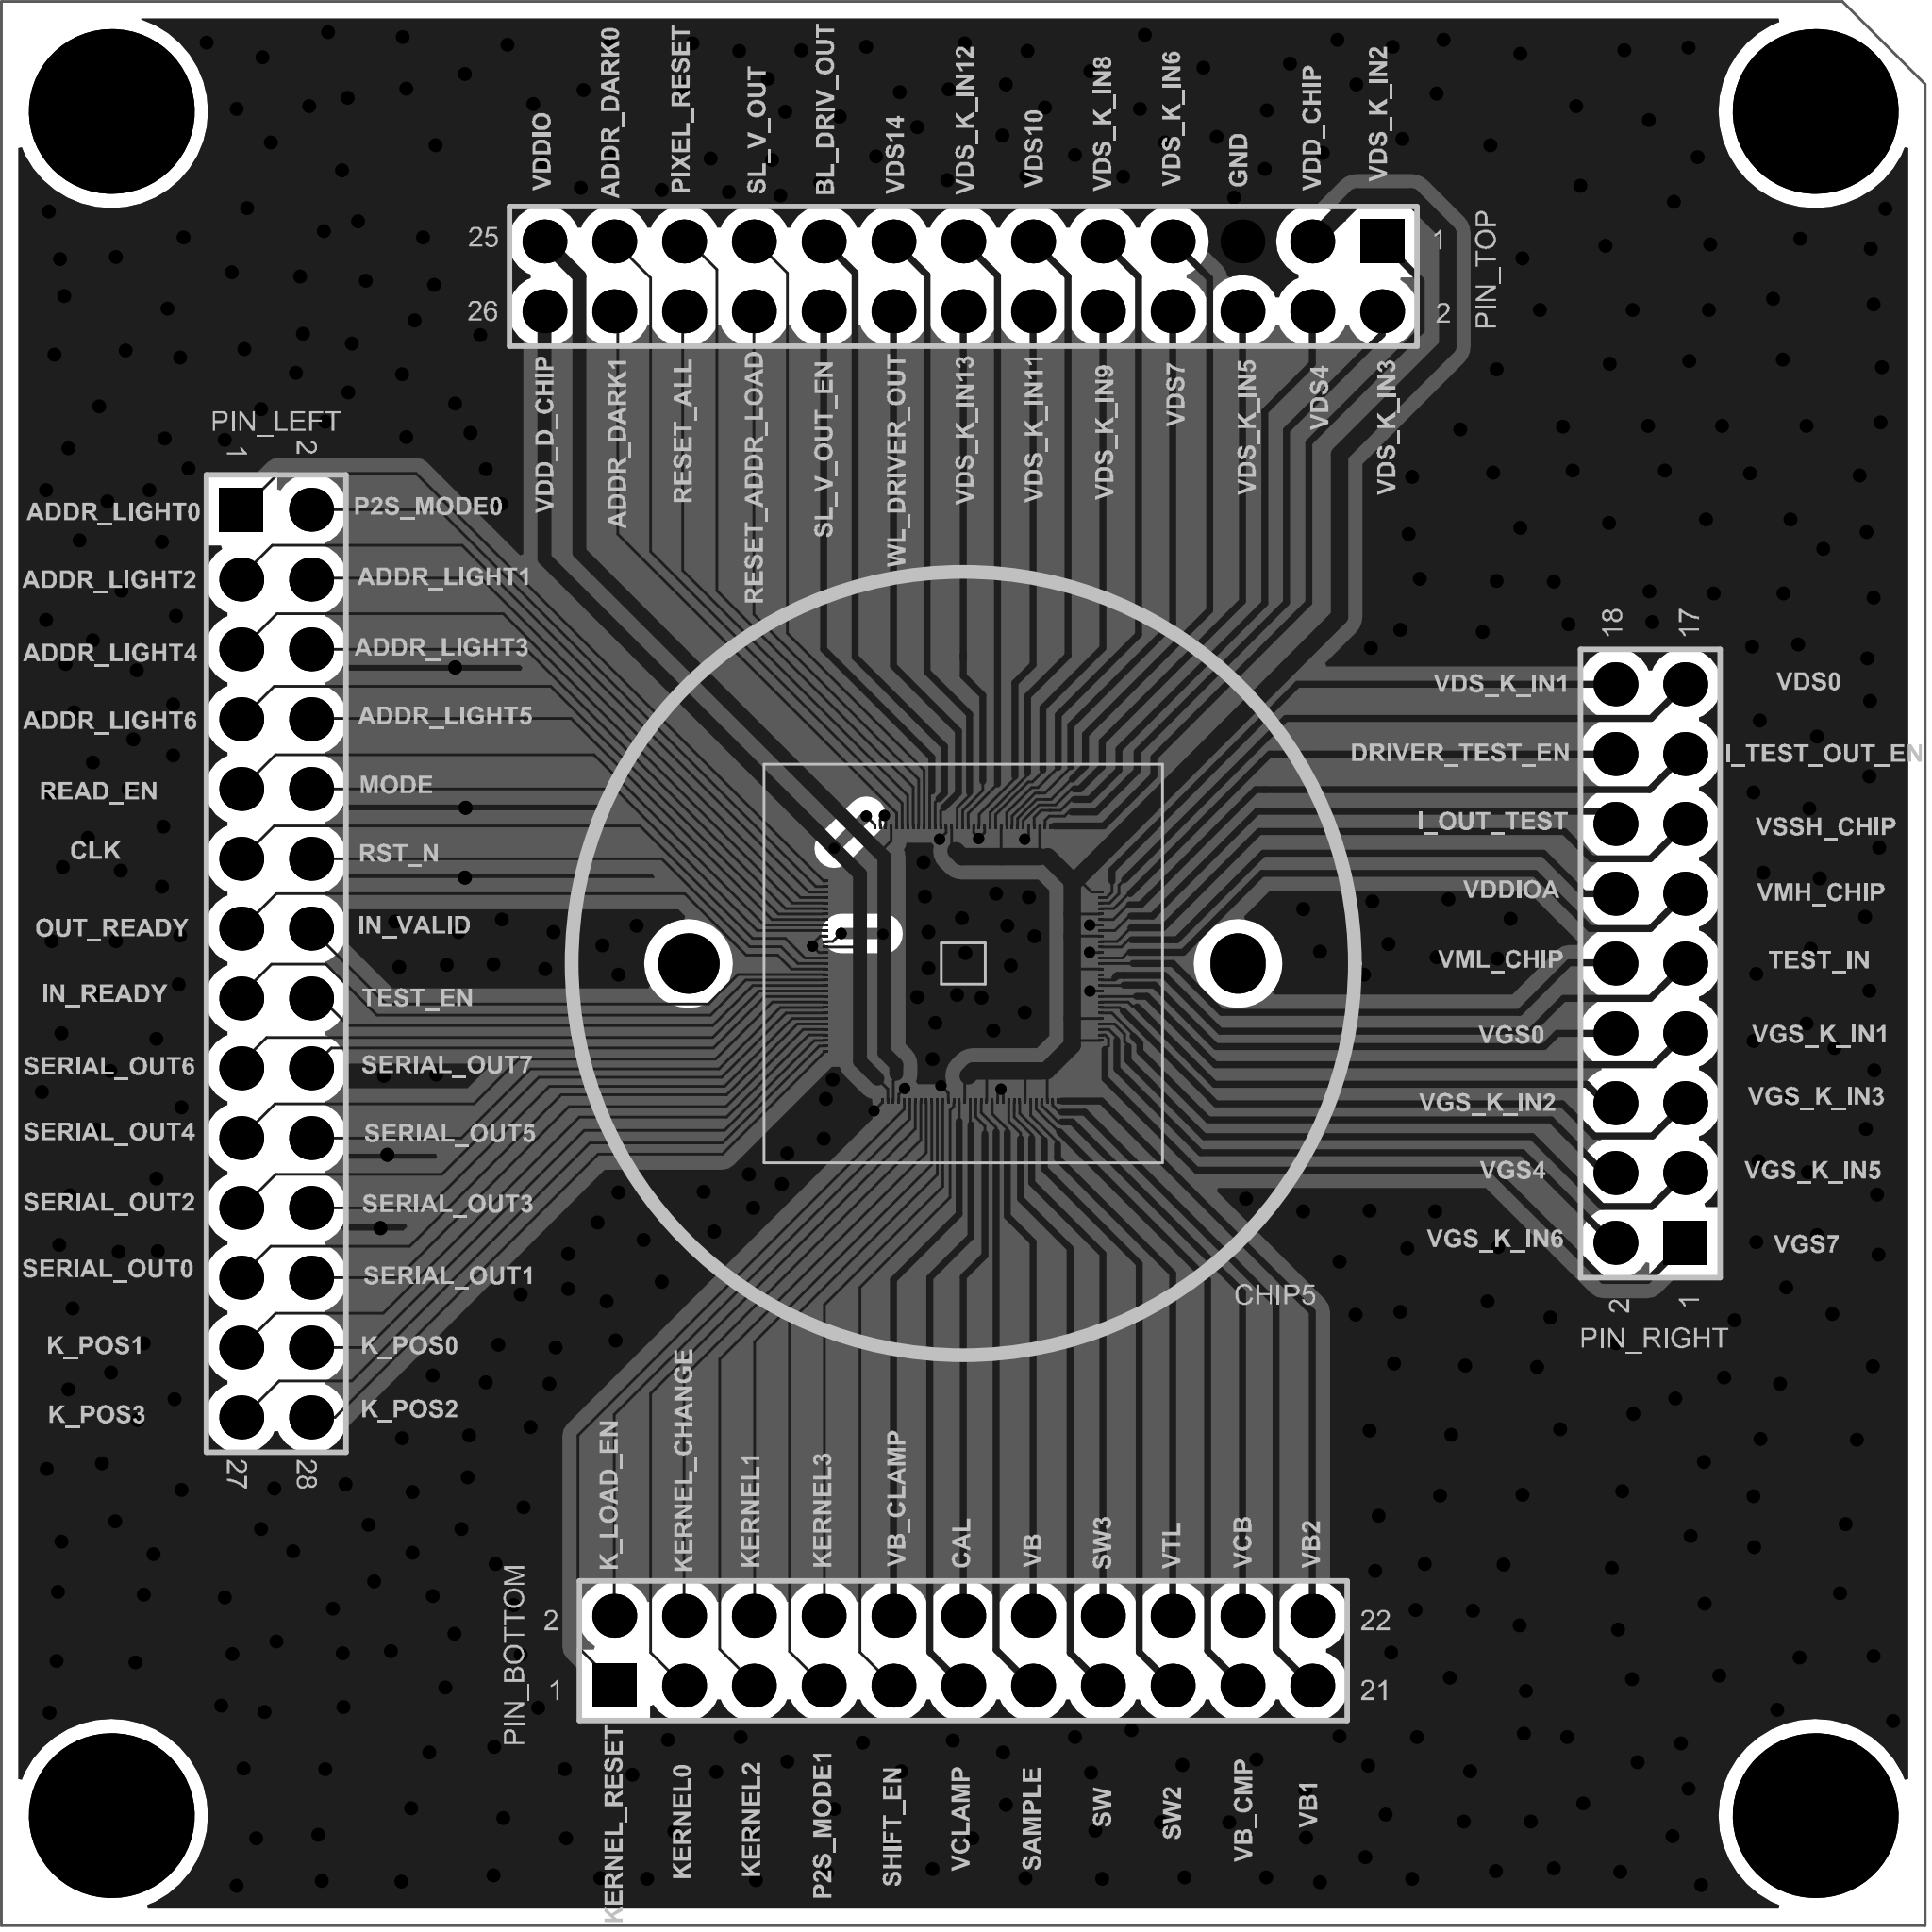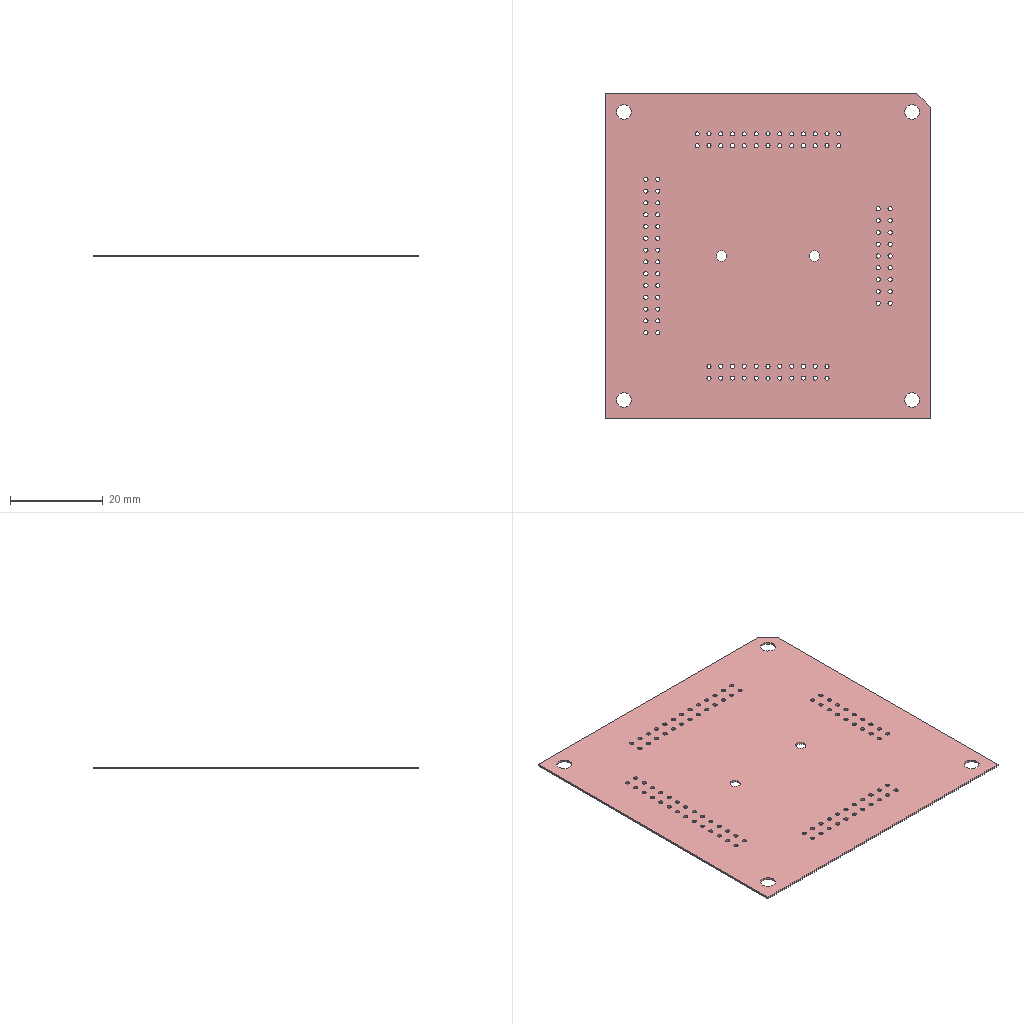Circuit board layout | Altium Designer | box 70 x 70 x 0.4 mm
Layer stack:
# Altium Designer layer stack of  (unit mm; dielectric type: 0 none, 1 core, 2 prepreg, 3 surface material)
index,name,kind,layer,copper_thickness_mm,dielectric_type,dielectric_thickness_mm,dielectric_material,dielectric_constant
0,Top Paste Mask Layer,other,,,,,,
1,Top Silkscreen Layer,other,,,,,,
2,Top Solder Mask Layer,dielectric,,,3,0.0102,Solder Resist,3.5
3,Top Layer,copper,Top Layer,0.0356,,,,
4,Dielectric1,dielectric,,,0,0.32,FR-4,4.8
5,Bottom Layer,copper,Bottom Layer,0.0356,,,,
6,Bottom Solder Mask Layer,dielectric,,,3,0.0102,Solder Resist,3.5
7,Bottom Silkscreen Layer,other,,,,,,
8,Bottom Paste Mask Layer,other,,,,,,
# drill layer pairs: low layer,high layer
drill_pair,Top Layer,Bottom Layer
Part placement:
Designator,Comment,Layer,Footprint,Center-X(mm),Center-Y(mm),Rotation
PIN_TOP,#NAME?,TopLayer,HDR2.54-LI-2X13P,35,60,180
PIN_RIGHT,#NAME?,TopLayer,HDR2.54-LI-2X9P,60,35,90
PIN_LEFT,#NAME?,TopLayer,HDR2.54-LI-2X14P,10,35,270
PIN_BOTTOM,#NAME?,TopLayer,HDR2.54-LI-2X11P,35,10,0
CHIP5,chip5,TopLayer,JSZ,35,35,0
Pad and via stacks:
# Altium Designer via and pad stacks of  (unit mm). Each distinct definition once, with the count of objects using it.
# via: kind,start_layer,end_layer,hole_mm,diameter_mm,mode(0 simple;1 top-mid-bottom;2 full stack),diameter_per_layer,count,example_net
# pad: kind,layer,hole_mm,hole_type(0 round;1 square;2 slot),plating,top_size,top_shape(1 round;2 rect;3 octagon;9 rounded rect),mid_size,bottom_size,mode,footprint,size_per_layer,count,example
pad,Multi-Layer,2.2,0,unplated,2.2x2.2,1,2.2x2.2,2.2x2.2,0,JSZ,,1,CHIP5.0
pad,Multi-Layer,2.2,0,unplated,2x2.2,1,2x2.2,2x2.2,0,JSZ,,1,CHIP5.0
pad,Multi-Layer,0.9,0,plated,1.6x1.6,2,1.6x1.6,1.6x1.6,0,HDR2.54-LI-2X14P,,1,PIN_LEFT.1
pad,Multi-Layer,0.9,0,plated,1.6x1.6,1,1.6x1.6,1.6x1.6,0,HDR2.54-LI-2X14P,,27,PIN_LEFT.2
pad,Multi-Layer,0.9,0,plated,1.6x1.6,2,1.6x1.6,1.6x1.6,0,HDR2.54-LI-2X13P,,1,PIN_TOP.1
pad,Multi-Layer,0.9,0,plated,1.6x1.6,1,1.6x1.6,1.6x1.6,0,HDR2.54-LI-2X13P,,25,PIN_TOP.2
pad,Multi-Layer,0.9,0,plated,1.6x1.6,1,1.6x1.6,1.6x1.6,0,HDR2.54-LI-2X11P,,21,PIN_BOTTOM.22
pad,Multi-Layer,0.9,0,plated,1.6x1.6,2,1.6x1.6,1.6x1.6,0,HDR2.54-LI-2X11P,,1,PIN_BOTTOM.1
pad,Multi-Layer,0.9,0,plated,1.6x1.6,1,1.6x1.6,1.6x1.6,0,HDR2.54-LI-2X9P,,17,PIN_RIGHT.16
pad,Multi-Layer,0.9,0,plated,1.6x1.6,2,1.6x1.6,1.6x1.6,0,HDR2.54-LI-2X9P,,1,PIN_RIGHT.1
pad,Multi-Layer,3.2,0,plated,6x6,1,6x6,6x6,0,,,4,0
pad,Top Layer,0,0,plated,0.1x0.2,2,0.1x0.2,0.1x0.2,0,JSZ,,126,CHIP5.98
via,Top Layer,Bottom Layer,0.2032,0.4064,0,,16,VDD_D_CHIP
via,Top Layer,Bottom Layer,0.3048,0.508,0,,464,GND
Copper pours:
name,layer,net,type(0 solid;1 hatched;2 none)
Bottom Layer-No Net,Bottom Layer,GND,0
Bottom Layer-No Net,Top Layer,GND,0
Design rules, without the lines most boards share:
# Altium Designer design rules of  (exported by Altium Designer, unit mm)
# columns: name | kind | enabled | priority | scope1 | scope2 | descriptor | typed fields (field=value)
Clearance | 0 | enabled | 3 | All | All | Clearance Constraint (Gap=3.95mil) (All),(All) | gap=0.1003
PlaneConnect | 6 | enabled | 1 | All | All | Power Plane Connect Rule(Direct Connect )(Expansion=20mil) (Conductor Width=10mil) (Air Gap=10mil) (Entries=4) (All) | relief_conductor_width=0.254 relief_entries=4 relief_expansion=0.508
PolygonConnect | 20 | enabled | 1 | All | All | Polygon Connect Rule(Direct Connect )(Conductor Width=10mil) (Relief Angle=90 Angle) (Entries=4) (Air Gap Width=10mil) (All),(All) | connect_style(0=relief,1=direct,2=none)=1 relief_conductor_width=0.254 relief_entries=4
Width | 2 | enabled | 1 | All | All | Width Constraint (Min=3.9mil) (Max=40mil) (Preferred=4mil) (All) |
RoutingVias | 11 | enabled | 1 | All | All | Routing Via (MinHoleWidth=8mil) (MaxHoleWidth=12mil) (PreferredHoleWidth=8mil) (MinWidth=16mil) (MaxWidth=20mil) (PreferedWidth=16mil) (All) | via_min_hole=0.2032 via_max_hole=0.3048 via_preferred_diameter=0.4064 via_preferred_hole=0.2032
PasteMaskExpansion | 14 | enabled | 1 | All | All | Paste Mask Expansion (Expansion =0mil) (All) | expansion=0
SolderMaskExpansion | 13 | enabled | 1 | All | All | Solder Mask Expansion (Expansion =4mil) (All) | expansion=0.1016
HoleSize | 42 | enabled | 1 | All | All | Hole Size Constraint (Min=1mil) (Max=500mil) (All) |
DiffPairsRouting | 51 | enabled | 1 | All | All | Differential Pairs Uncoupled Length using the Gap Constraints (Min=10mil) (Max=10mil) (Prefered=10mil)  and Width Constraints (Min=15mil) (Max=15mil) (Prefered=15mil) (All) |
HoleToHoleClearance | 52 | enabled | 1 | All | All | Hole To Hole Clearance (Gap=0mil) (All),(All) | gap=0
MinimumSolderMaskSliver | 53 | enabled | 1 | All | All | Minimum Solder Mask Sliver (Gap=0mil) (All),(All) |
SilkscreenOverComponentPads | 54 | enabled | 1 | IsPad | All | Silk To Solder Mask (Clearance=0mil) (IsPad),(All) |
SilkToSilkClearance | 55 | enabled | 1 | All | All | Silk to Silk (Clearance=0mil) (All),(All) |
Clearance_1 | 0 | enabled | 2 | ispad | ispad | Clearance Constraint (Gap=3.9mil) (ispad),(ispad) | gap=0.0991
Clearance_2 | 0 | enabled | 1 | INPOLYGON | All | Clearance Constraint (Gap=20mil) (INPOLYGON),(All) | gap=0.508
Classes set for this board:
# Altium Designer classes of  (member kind: 0 net, 1 component, 2 from-to, 3 pad, 4 layer, 5 differential pair, 6 design channel, 7 polygon, 8 structure, 9 xSignal)
# columns: class name | member kind | superclass | members
1_P1.schdoc | 1 | no | CHIP5; Pin_Bottom; Pin_Left; Pin_Right; pin_Top;